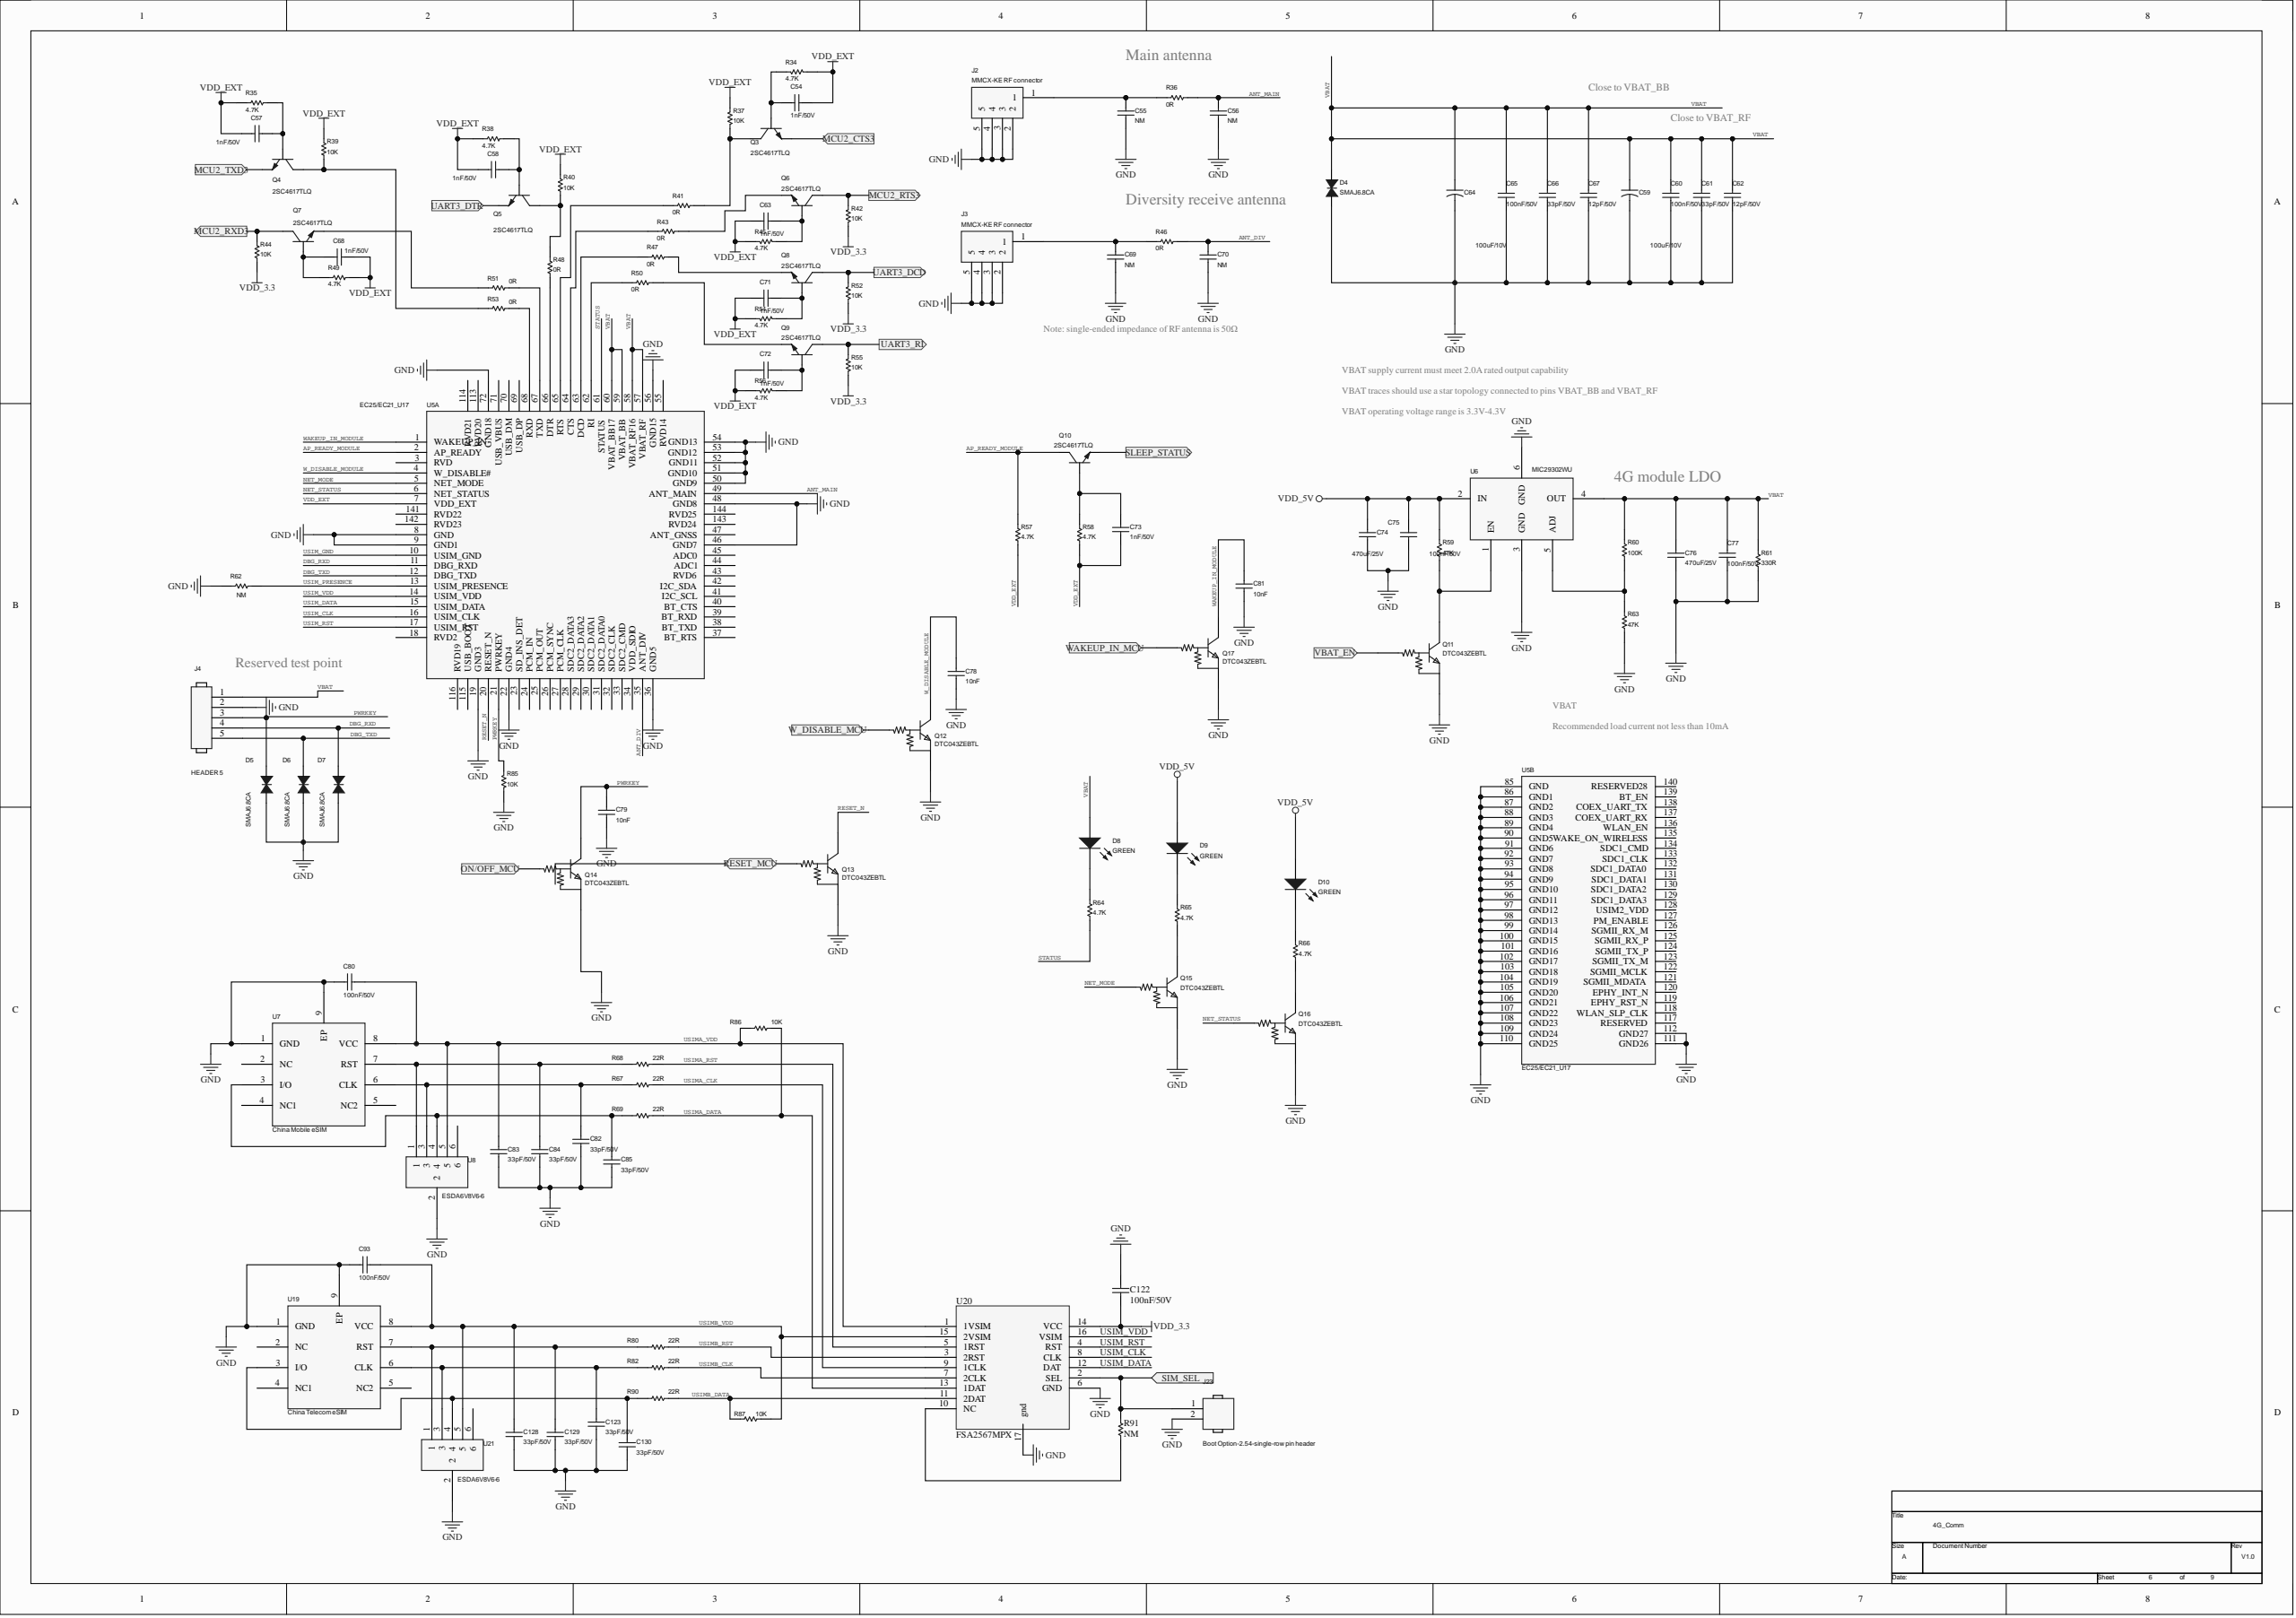Circuit board | Altium Designer | 313 parts | 216 nets | one sheet of the schematic
Parts on this sheet (reference | value | footprint):
C54 | 1nF/50V | C0603
C55 | NM | C0603
C56 | NM | C0603
C57 | 1nF/50V | C0603
C58 | 1nF/50V | C0603
C59 | 100uF/10V | RB5*7
C60 | 100nF/50V | C0603
C61 | 33pF/50V | C0603
C62 | 12pF/50V | C0603
C63 | 1nF/50V | C0603
C64 | 100uF/10V | RB5*7
C65 | 100nF/50V | C0603
C66 | 33pF/50V | C0603
C67 | 12pF/50V | C0603
C68 | 1nF/50V | C0603
C69 | NM | C0603
C70 | NM | C0603
C71 | 1nF/50V | C0603
C72 | 1nF/50V | C0603
C73 | 1nF/50V | C0603
C74 | 470uF/25V | RB8*11_5
C75 | 100nF/50V | C0603
C76 | 470uF/25V | RB8*11_5
C77 | 100nF/50V | C0603
C78 | 10nF | C0603
C79 | 10nF | C0603
C80 | 100nF/50V | C0603
C81 | 10nF | C0603
C82 | 33pF/50V | C0603
C83 | 33pF/50V | C0603
C84 | 33pF/50V | C0603
C85 | 33pF/50V | C0603
C93 | 100nF/50V | C0603
C122 | 100nF/50V | C0603
C123 | 33pF/50V | C0603
C128 | 33pF/50V | C0603
C129 | 33pF/50V | C0603
C130 | 33pF/50V | C0603
D4 | SMAJ6.8CA | SMA
D5 | SMAJ6.8CA | SMA
D6 | SMAJ6.8CA | SMA
D7 | SMAJ6.8CA | SMA
D8 | GREEN | LED0805
D9 | GREEN | LED0805
D10 | GREEN | LED0805
J2 | MMCX-KE RF connector | MMCX-KE
J3 | MMCX-KE RF connector | MMCX-KE
J4 | HEADER 5 | 2.54mm_paizhen_5pin
J23 | Boot Option-2.54-single-row pin header | HDR_1X2_254
Q3 | 2SC4617TLQ | EMT3
Q4 | 2SC4617TLQ | EMT3
Q5 | 2SC4617TLQ | EMT3
Q6 | 2SC4617TLQ | EMT3
Q7 | 2SC4617TLQ | EMT3
Q8 | 2SC4617TLQ | EMT3
Q9 | 2SC4617TLQ | EMT3
Q10 | 2SC4617TLQ | EMT3
Q11 | DTC043ZEBTL | SOT-416_L1_6-W0_8-P1_00-LS1_6-BR
Q12 | DTC043ZEBTL | SOT-416_L1_6-W0_8-P1_00-LS1_6-BR
Q13 | DTC043ZEBTL | SOT-416_L1_6-W0_8-P1_00-LS1_6-BR
Q14 | DTC043ZEBTL | SOT-416_L1_6-W0_8-P1_00-LS1_6-BR
Q15 | DTC043ZEBTL | SOT-416_L1_6-W0_8-P1_00-LS1_6-BR
Q16 | DTC043ZEBTL | SOT-416_L1_6-W0_8-P1_00-LS1_6-BR
Q17 | DTC043ZEBTL | SOT-416_L1_6-W0_8-P1_00-LS1_6-BR
R34 | 4.7K | R0603
R35 | 4.7K | R0603
R36 | 0R | R0603
R37 | 10K | R0603
R38 | 4.7K | R0603
R39 | 10K | R0603
R40 | 10K | R0603
R41 | 0R | R0603
R42 | 10K | R0603
R43 | 0R | R0603
R44 | 10K | R0603
R45 | 4.7K | R0603
R46 | 0R | R0603
R47 | 0R | R0603
R48 | 0R | R0603
R49 | 4.7K | R0603
R50 | 0R | R0603
R51 | 0R | R0603
R52 | 10K | R0603
R53 | 0R | R0603
R54 | 4.7K | R0603
R55 | 10K | R0603
R56 | 4.7K | R0603
R57 | 4.7K | R0603
R58 | 4.7K | R0603
R59 | 47K | R0603
R60 | 100K | R0603
R61 | 330R | R0603
R62 | NM | R0603
R63 | 47K | R0603
R64 | 4.7K | R0603
R65 | 4.7K | R0603
R66 | 4.7K | R0603
R67 | 22R | R0603
R68 | 22R | R0603
R69 | 22R | R0603
R80 | 22R | R0603
R82 | 22R | R0603
R85 | 10K | R0603
R86 | 10K | R0603
R87 | 10K | R0603
R90 | 22R | R0603
R91 | NM | R0603
U5 | EC25/EC21_U17 | EC20
U6 | MIC29302WU | TO-263-5
U7 | China Mobile eSIM | DFN-8_L6.0-W5.0-P1.27-BL-EP-A
U8 | ESDA6V8V6-6 | SOT-563
U19 | China Telecom eSIM | DFN-8_L6.0-W5.0-P1.27-BL-EP-A
U20 | FSA2567MPX | TQFN-16_L3.0-W3.0-P0.50-BL-EP1.7
U21 | ESDA6V8V6-6 | SOT-563
Nets of these parts (net: part-pin ...):
WAKEUP_IN_MODULE: C81-1 Q17-3 U5-1
W_DISABLE_MODULE: C78-1 Q12-3 U5-4
VDD_EXT: C54-1 C57-1 C58-1 C63-2 C68-2 C71-2 C72-2 C73-2 R34-2 R35-2 R37-1 R38-2 R39-1 R40-1 R45-1 R49-1 R54-1 R56-1 R57-1 R58-1 U5-7
VDD_5V: C74-1 C75-1 D9-1 D10-1 R59-2 U6-2
VDD_3.3: C122-2 R42-2 R44-2 R52-2 R55-2 U20-14
VBAT: C59-1 C60-1 C61-1 C62-1 C64-1 C65-1 C66-1 C67-1 C76-1 C77-1 D4-2 D8-1 J4-1 R60-2 R61-2 U6-4 U5-57 U5-58 U5-59 U5-60
USIMB_VDD: C93-1 C128-1 R87-1 U19-8 U20-15 U21-5
USIMB_RST: R80-1 U20-3
USIMB_DATA: R87-2 R90-1 U20-11
USIMB_CLK: R82-1 U20-7
USIMA_VDD: C80-1 C83-1 R86-2 U7-8 U8-5 U20-1
USIMA_RST: R68-1 U20-5
USIMA_DATA: R69-1 R86-1 U20-13
USIMA_CLK: R67-1 U20-9
USIM_VDD: U20-16 U5-14
USIM_RST: U20-4 U5-17
USIM_PRESENCE: R62-2 U5-13
USIM_DATA: U20-12 U5-15
USIM_CLK: U20-8 U5-16
STATUS: R64-2 U5-61
RESET_N: Q13-3 U5-20
PWRKEY: C79-1 D5-2 J4-3 Q14-3 R85-1 U5-21
NetR91_2: R91-2 U20-10
NetR60_1: R60-1 R63-2 U6-5
NetR53_2: R53-2 U5-68
NetR51_2: R51-2 U5-67
NetR50_2: R50-2 U5-62
NetR48_2: R48-2 U5-66
NetR47_2: R47-2 U5-63
NetR43_2: R43-2 U5-64
NetR41_2: R41-2 U5-65
NetQ17_1: Q17-1
NetQ16_3: Q16-3 R66-2
NetQ15_3: Q15-3 R65-2
NetQ14_1: Q14-1
NetQ13_1: Q13-1
NetQ12_1: Q12-1
NetQ11_3: Q11-3 R59-1 U6-1
NetQ11_1: Q11-1
NetQ10_1: Q10-1
NetQ9_3: Q9-3 R55-1
NetQ9_1: Q9-1 R50-1
NetQ8_3: Q8-3 R52-1
NetQ8_1: Q8-1 R47-1
NetQ7_1: Q7-1 R51-1
NetQ6_3: Q6-3 R42-1
NetQ6_1: Q6-1 R43-1
NetQ5_3: Q5-3 R40-2 R48-1
NetQ5_1: Q5-1
NetQ4_3: Q4-3 R39-2 R53-1
NetQ3_3: Q3-3 R37-2 R41-1
NetQ3_1: Q3-1
NetJ23_1: J23-1 R91-1 U20-2
NetJ17_2: Q7-3 R44-1
NetJ17_1: Q4-1
NetD10_2: D10-2 R66-1
NetD9_2: D9-2 R65-1
NetD8_2: D8-2 R64-1
NetC130_1: C130-1 R90-2 U19-3 U21-4
NetC129_1: C129-1 R80-2 U19-7 U21-1
NetC123_1: C123-1 R82-2 U19-6 U21-3
NetC85_1: C85-1 R69-2 U7-3 U8-4
NetC84_1: C84-1 R68-2 U7-7 U8-1
NetC82_1: C82-1 R67-2 U7-6 U8-3
NetC73_1: C73-1 Q10-2 R58-2
NetC72_1: C72-1 Q9-2 R56-2
NetC71_1: C71-1 Q8-2 R54-2
NetC69_2: C69-2 J3-1 R46-2
NetC68_1: C68-1 Q7-2 R49-2
NetC63_1: C63-1 Q6-2 R45-2
NetC58_2: C58-2 Q5-2 R38-1
NetC57_2: C57-2 Q4-2 R35-1
NetC55_2: C55-2 J2-1 R36-2
NetC54_2: C54-2 Q3-2 R34-1
NET_STATUS: Q16-1 U5-6
NET_MODE: Q15-1 U5-5
GND: C55-1 C56-1 C59-2 C60-2 C61-2 C62-2 C64-2 C65-2 C66-2 C67-2 C69-1 C70-1 C74-2 C75-2 C76-2 C77-2 C78-2 C79-2 C80-2 C81-2 C82-2 C83-2 C84-2 C85-2 C93-2 C122-1 C123-2 C128-2 C129-2 C130-2 D4-1 D5-1 D6-1 D7-1 J2-2 J2-3 J2-4 J2-5 J3-2 J3-3 J3-4 J3-5 J4-2 J23-2 Q11-2 Q12-2 Q13-2 Q14-2 Q15-2 Q16-2 Q17-2 R61-1 R62-1 R63-1 R85-2 U6-3 U6-6 U7-1 U7-9 U8-2 U19-1 U19-9 U20-6 U20-17 U21-2 U5-8 U5-9 U5-19 U5-22 U5-36 U5-46 U5-48 U5-50 U5-51 U5-52 U5-53 U5-54 U5-56 U5-72 U5-85 U5-86 U5-87 U5-88 U5-89 U5-90 U5-91 U5-92 U5-93 U5-94 U5-95 U5-96 U5-97 U5-98 U5-99 U5-100 U5-101 U5-102 U5-103 U5-104 U5-105 U5-106 U5-107 U5-108 U5-109 U5-110 U5-111 U5-112
DBG_TXD: D6-2 J4-5 U5-12
DBG_RXD: D7-2 J4-4 U5-11
AP_READY_MODULE: Q10-3 R57-2 U5-2
ANT_MAIN: C56-2 R36-1 U5-49
ANT_DIV: C70-2 R46-1 U5-35